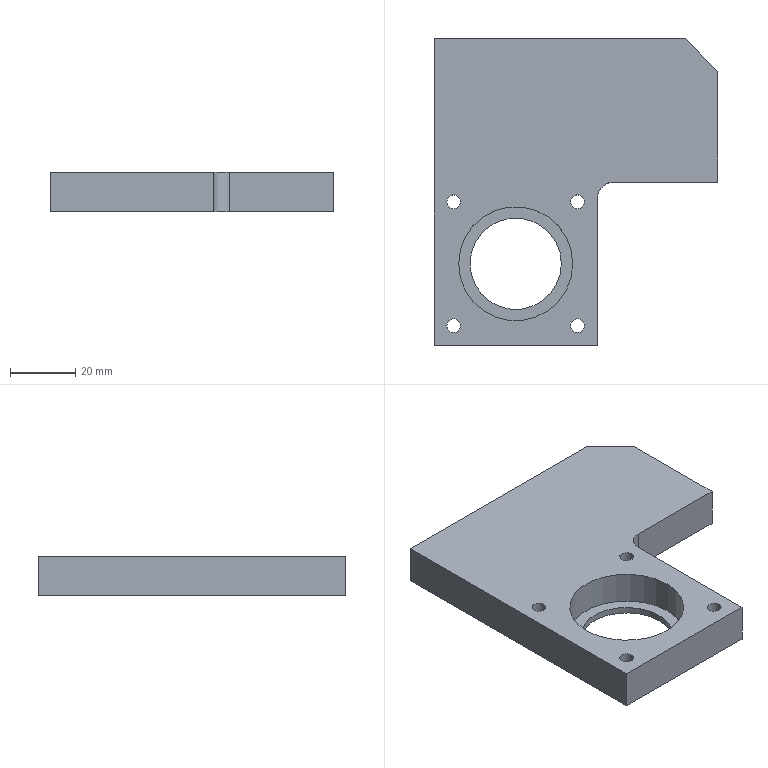Part | SolidWorks | features MirrorStock 1 | 1 solid | 47 faces | box 87 x 94 x 12 mm | volume 62817 mm3 | cylinder 25 | cone 12 | plane 10 | commonest cylinder face diameters 4.2 x20 28 x2 35 x2 10 x1
STEP:
#1=CARTESIAN_POINT('',(22.1,28.5,2.1));
#2=VERTEX_POINT('',#1);
#3=CARTESIAN_POINT('',(22.1,28.5,-2.1));
#4=VERTEX_POINT('',#3);
#5=CARTESIAN_POINT('',(22.1,28.5,0.));
#6=DIRECTION('',(-1.,0.,0.));
#7=DIRECTION('',(0.,0.,1.));
#8=AXIS2_PLACEMENT_3D('',#5,#6,#7);
#9=CIRCLE('',#8,2.1);
#10=EDGE_CURVE('',#2,#4,#9,.T.);
#11=ORIENTED_EDGE('',*,*,#10,.T.);
#12=CARTESIAN_POINT('',(34.5,28.5,-2.1));
#13=VERTEX_POINT('',#12);
#14=CARTESIAN_POINT('',(34.5,28.5,-2.1));
#15=DIRECTION('',(1.,0.,0.));
#16=VECTOR('',#15,1000.);
#17=LINE('',#14,#16);
#18=EDGE_CURVE('',#4,#13,#17,.T.);
#19=ORIENTED_EDGE('',*,*,#18,.T.);
#20=CARTESIAN_POINT('',(34.5,28.5,2.1));
#21=VERTEX_POINT('',#20);
#22=CARTESIAN_POINT('',(34.5,28.5,0.));
#23=DIRECTION('',(-1.,0.,0.));
#24=DIRECTION('',(0.,0.,1.));
#25=AXIS2_PLACEMENT_3D('',#22,#23,#24);
#26=CIRCLE('',#25,2.1);
#27=EDGE_CURVE('',#21,#13,#26,.T.);
#28=ORIENTED_EDGE('',*,*,#27,.F.);
#29=CARTESIAN_POINT('',(34.5,28.5,2.1));
#30=DIRECTION('',(1.,0.,0.));
#31=VECTOR('',#30,1000.);
#32=LINE('',#29,#31);
#33=EDGE_CURVE('',#2,#21,#32,.T.);
#34=ORIENTED_EDGE('',*,*,#33,.F.);
#35=EDGE_LOOP('',(#11,#19,#28,#34));
#36=FACE_OUTER_BOUND('',#35,.T.);
#37=CARTESIAN_POINT('',(34.5,28.5,0.));
#38=DIRECTION('',(1.,0.,0.));
#39=DIRECTION('',(0.,0.,1.));
#40=AXIS2_PLACEMENT_3D('',#37,#38,#39);
#41=CYLINDRICAL_SURFACE('',#40,2.1);
#42=ADVANCED_FACE('',(#36),#41,.F.);
#43=CARTESIAN_POINT('',(20.838,28.5,0.));
#44=VERTEX_POINT('',#43);
#45=CARTESIAN_POINT('',(22.1,28.5,2.1));
#46=DIRECTION('',(0.515,0.,0.8572));
#47=VECTOR('',#46,1000.);
#48=LINE('',#45,#47);
#49=EDGE_CURVE('',#44,#2,#48,.T.);
#50=ORIENTED_EDGE('',*,*,#49,.F.);
#51=CARTESIAN_POINT('',(22.1,28.5,-2.1));
#52=DIRECTION('',(0.515,0.,-0.8572));
#53=VECTOR('',#52,1000.);
#54=LINE('',#51,#53);
#55=EDGE_CURVE('',#44,#4,#54,.T.);
#56=ORIENTED_EDGE('',*,*,#55,.T.);
#57=ORIENTED_EDGE('',*,*,#10,.F.);
#58=EDGE_LOOP('',(#50,#56,#57));
#59=FACE_OUTER_BOUND('',#58,.T.);
#60=CARTESIAN_POINT('',(22.1,28.5,0.));
#61=DIRECTION('',(1.,0.,0.));
#62=DIRECTION('',(0.,0.,1.));
#63=AXIS2_PLACEMENT_3D('',#60,#61,#62);
#64=CONICAL_SURFACE('',#63,2.1,1.03);
#65=ADVANCED_FACE('',(#59),#64,.F.);
#66=CARTESIAN_POINT('',(22.1,10.5,2.1));
#67=VERTEX_POINT('',#66);
#68=CARTESIAN_POINT('',(22.1,10.5,-2.1));
#69=VERTEX_POINT('',#68);
#70=CARTESIAN_POINT('',(22.1,10.5,0.));
#71=DIRECTION('',(-1.,0.,0.));
#72=DIRECTION('',(0.,0.,1.));
#73=AXIS2_PLACEMENT_3D('',#70,#71,#72);
#74=CIRCLE('',#73,2.1);
#75=EDGE_CURVE('',#67,#69,#74,.T.);
#76=ORIENTED_EDGE('',*,*,#75,.T.);
#77=CARTESIAN_POINT('',(34.5,10.5,-2.1));
#78=VERTEX_POINT('',#77);
#79=CARTESIAN_POINT('',(34.5,10.5,-2.1));
#80=DIRECTION('',(1.,0.,0.));
#81=VECTOR('',#80,1000.);
#82=LINE('',#79,#81);
#83=EDGE_CURVE('',#69,#78,#82,.T.);
#84=ORIENTED_EDGE('',*,*,#83,.T.);
#85=CARTESIAN_POINT('',(34.5,10.5,2.1));
#86=VERTEX_POINT('',#85);
#87=CARTESIAN_POINT('',(34.5,10.5,0.));
#88=DIRECTION('',(-1.,0.,0.));
#89=DIRECTION('',(0.,0.,1.));
#90=AXIS2_PLACEMENT_3D('',#87,#88,#89);
#91=CIRCLE('',#90,2.1);
#92=EDGE_CURVE('',#86,#78,#91,.T.);
#93=ORIENTED_EDGE('',*,*,#92,.F.);
#94=CARTESIAN_POINT('',(34.5,10.5,2.1));
#95=DIRECTION('',(1.,0.,0.));
#96=VECTOR('',#95,1000.);
#97=LINE('',#94,#96);
#98=EDGE_CURVE('',#67,#86,#97,.T.);
#99=ORIENTED_EDGE('',*,*,#98,.F.);
#100=EDGE_LOOP('',(#76,#84,#93,#99));
#101=FACE_OUTER_BOUND('',#100,.T.);
#102=CARTESIAN_POINT('',(34.5,10.5,0.));
#103=DIRECTION('',(1.,0.,0.));
#104=DIRECTION('',(0.,0.,1.));
#105=AXIS2_PLACEMENT_3D('',#102,#103,#104);
#106=CYLINDRICAL_SURFACE('',#105,2.1);
#107=ADVANCED_FACE('',(#101),#106,.F.);
#108=CARTESIAN_POINT('',(20.838,10.5,0.));
#109=VERTEX_POINT('',#108);
#110=CARTESIAN_POINT('',(22.1,10.5,2.1));
#111=DIRECTION('',(0.515,0.,0.8572));
#112=VECTOR('',#111,1000.);
#113=LINE('',#110,#112);
#114=EDGE_CURVE('',#109,#67,#113,.T.);
#115=ORIENTED_EDGE('',*,*,#114,.F.);
#116=CARTESIAN_POINT('',(22.1,10.5,-2.1));
#117=DIRECTION('',(0.515,0.,-0.8572));
#118=VECTOR('',#117,1000.);
#119=LINE('',#116,#118);
#120=EDGE_CURVE('',#109,#69,#119,.T.);
#121=ORIENTED_EDGE('',*,*,#120,.T.);
#122=ORIENTED_EDGE('',*,*,#75,.F.);
#123=EDGE_LOOP('',(#115,#121,#122));
#124=FACE_OUTER_BOUND('',#123,.T.);
#125=CARTESIAN_POINT('',(22.1,10.5,0.));
#126=DIRECTION('',(1.,0.,0.));
#127=DIRECTION('',(0.,0.,1.));
#128=AXIS2_PLACEMENT_3D('',#125,#126,#127);
#129=CONICAL_SURFACE('',#128,2.1,1.03);
#130=ADVANCED_FACE('',(#124),#129,.F.);
#131=CARTESIAN_POINT('',(12.5,34.1,-2.1));
#132=VERTEX_POINT('',#131);
#133=CARTESIAN_POINT('',(12.5,34.1,2.1));
#134=VERTEX_POINT('',#133);
#135=CARTESIAN_POINT('',(12.5,34.1,0.));
#136=DIRECTION('',(0.,-1.,0.));
#137=DIRECTION('',(0.,0.,-1.));
#138=AXIS2_PLACEMENT_3D('',#135,#136,#137);
#139=CIRCLE('',#138,2.1);
#140=EDGE_CURVE('',#132,#134,#139,.T.);
#141=ORIENTED_EDGE('',*,*,#140,.T.);
#142=CARTESIAN_POINT('',(12.5,46.5,2.1));
#143=VERTEX_POINT('',#142);
#144=CARTESIAN_POINT('',(12.5,46.5,2.1));
#145=DIRECTION('',(0.,1.,0.));
#146=VECTOR('',#145,1000.);
#147=LINE('',#144,#146);
#148=EDGE_CURVE('',#134,#143,#147,.T.);
#149=ORIENTED_EDGE('',*,*,#148,.T.);
#150=CARTESIAN_POINT('',(12.5,46.5,-2.1));
#151=VERTEX_POINT('',#150);
#152=CARTESIAN_POINT('',(12.5,46.5,0.));
#153=DIRECTION('',(0.,-1.,0.));
#154=DIRECTION('',(0.,0.,-1.));
#155=AXIS2_PLACEMENT_3D('',#152,#153,#154);
#156=CIRCLE('',#155,2.1);
#157=EDGE_CURVE('',#151,#143,#156,.T.);
#158=ORIENTED_EDGE('',*,*,#157,.F.);
#159=CARTESIAN_POINT('',(12.5,46.5,-2.1));
#160=DIRECTION('',(0.,1.,0.));
#161=VECTOR('',#160,1000.);
#162=LINE('',#159,#161);
#163=EDGE_CURVE('',#132,#151,#162,.T.);
#164=ORIENTED_EDGE('',*,*,#163,.F.);
#165=EDGE_LOOP('',(#141,#149,#158,#164));
#166=FACE_OUTER_BOUND('',#165,.T.);
#167=CARTESIAN_POINT('',(12.5,46.5,0.));
#168=DIRECTION('',(0.,1.,0.));
#169=DIRECTION('',(0.,0.,-1.));
#170=AXIS2_PLACEMENT_3D('',#167,#168,#169);
#171=CYLINDRICAL_SURFACE('',#170,2.1);
#172=ADVANCED_FACE('',(#166),#171,.F.);
#173=CARTESIAN_POINT('',(12.5,32.838,0.));
#174=VERTEX_POINT('',#173);
#175=CARTESIAN_POINT('',(12.5,34.1,-2.1));
#176=DIRECTION('',(0.,0.515,-0.8572));
#177=VECTOR('',#176,1000.);
#178=LINE('',#175,#177);
#179=EDGE_CURVE('',#174,#132,#178,.T.);
#180=ORIENTED_EDGE('',*,*,#179,.F.);
#181=CARTESIAN_POINT('',(12.5,34.1,2.1));
#182=DIRECTION('',(0.,0.515,0.8572));
#183=VECTOR('',#182,1000.);
#184=LINE('',#181,#183);
#185=EDGE_CURVE('',#174,#134,#184,.T.);
#186=ORIENTED_EDGE('',*,*,#185,.T.);
#187=ORIENTED_EDGE('',*,*,#140,.F.);
#188=EDGE_LOOP('',(#180,#186,#187));
#189=FACE_OUTER_BOUND('',#188,.T.);
#190=CARTESIAN_POINT('',(12.5,34.1,0.));
#191=DIRECTION('',(0.,1.,0.));
#192=DIRECTION('',(0.,0.,-1.));
#193=AXIS2_PLACEMENT_3D('',#190,#191,#192);
#194=CONICAL_SURFACE('',#193,2.1,1.03);
#195=ADVANCED_FACE('',(#189),#194,.F.);
#196=CARTESIAN_POINT('',(-7.5,34.1,-2.1));
#197=VERTEX_POINT('',#196);
#198=CARTESIAN_POINT('',(-7.5,34.1,2.1));
#199=VERTEX_POINT('',#198);
#200=CARTESIAN_POINT('',(-7.5,34.1,0.));
#201=DIRECTION('',(0.,-1.,0.));
#202=DIRECTION('',(0.,0.,-1.));
#203=AXIS2_PLACEMENT_3D('',#200,#201,#202);
#204=CIRCLE('',#203,2.1);
#205=EDGE_CURVE('',#197,#199,#204,.T.);
#206=ORIENTED_EDGE('',*,*,#205,.T.);
#207=CARTESIAN_POINT('',(-7.5,46.5,2.1));
#208=VERTEX_POINT('',#207);
#209=CARTESIAN_POINT('',(-7.5,46.5,2.1));
#210=DIRECTION('',(0.,1.,0.));
#211=VECTOR('',#210,1000.);
#212=LINE('',#209,#211);
#213=EDGE_CURVE('',#199,#208,#212,.T.);
#214=ORIENTED_EDGE('',*,*,#213,.T.);
#215=CARTESIAN_POINT('',(-7.5,46.5,-2.1));
#216=VERTEX_POINT('',#215);
#217=CARTESIAN_POINT('',(-7.5,46.5,0.));
#218=DIRECTION('',(0.,-1.,0.));
#219=DIRECTION('',(0.,0.,-1.));
#220=AXIS2_PLACEMENT_3D('',#217,#218,#219);
#221=CIRCLE('',#220,2.1);
#222=EDGE_CURVE('',#216,#208,#221,.T.);
#223=ORIENTED_EDGE('',*,*,#222,.F.);
#224=CARTESIAN_POINT('',(-7.5,46.5,-2.1));
#225=DIRECTION('',(0.,1.,0.));
#226=VECTOR('',#225,1000.);
#227=LINE('',#224,#226);
#228=EDGE_CURVE('',#197,#216,#227,.T.);
#229=ORIENTED_EDGE('',*,*,#228,.F.);
#230=EDGE_LOOP('',(#206,#214,#223,#229));
#231=FACE_OUTER_BOUND('',#230,.T.);
#232=CARTESIAN_POINT('',(-7.5,46.5,0.));
#233=DIRECTION('',(0.,1.,0.));
#234=DIRECTION('',(0.,0.,-1.));
#235=AXIS2_PLACEMENT_3D('',#232,#233,#234);
#236=CYLINDRICAL_SURFACE('',#235,2.1);
#237=ADVANCED_FACE('',(#231),#236,.F.);
#238=CARTESIAN_POINT('',(-7.5,32.838,0.));
#239=VERTEX_POINT('',#238);
#240=CARTESIAN_POINT('',(-7.5,34.1,-2.1));
#241=DIRECTION('',(0.,0.515,-0.8572));
#242=VECTOR('',#241,1000.);
#243=LINE('',#240,#242);
#244=EDGE_CURVE('',#239,#197,#243,.T.);
#245=ORIENTED_EDGE('',*,*,#244,.F.);
#246=CARTESIAN_POINT('',(-7.5,34.1,2.1));
#247=DIRECTION('',(0.,0.515,0.8572));
#248=VECTOR('',#247,1000.);
#249=LINE('',#246,#248);
#250=EDGE_CURVE('',#239,#199,#249,.T.);
#251=ORIENTED_EDGE('',*,*,#250,.T.);
#252=ORIENTED_EDGE('',*,*,#205,.F.);
#253=EDGE_LOOP('',(#245,#251,#252));
#254=FACE_OUTER_BOUND('',#253,.T.);
#255=CARTESIAN_POINT('',(-7.5,34.1,0.));
#256=DIRECTION('',(0.,1.,0.));
#257=DIRECTION('',(0.,0.,-1.));
#258=AXIS2_PLACEMENT_3D('',#255,#256,#257);
#259=CONICAL_SURFACE('',#258,2.1,1.03);
#260=ADVANCED_FACE('',(#254),#259,.F.);
#261=CARTESIAN_POINT('',(-27.5,34.1,-2.1));
#262=VERTEX_POINT('',#261);
#263=CARTESIAN_POINT('',(-27.5,34.1,2.1));
#264=VERTEX_POINT('',#263);
#265=CARTESIAN_POINT('',(-27.5,34.1,0.));
#266=DIRECTION('',(0.,-1.,0.));
#267=DIRECTION('',(0.,0.,-1.));
#268=AXIS2_PLACEMENT_3D('',#265,#266,#267);
#269=CIRCLE('',#268,2.1);
#270=EDGE_CURVE('',#262,#264,#269,.T.);
#271=ORIENTED_EDGE('',*,*,#270,.T.);
#272=CARTESIAN_POINT('',(-27.5,46.5,2.1));
#273=VERTEX_POINT('',#272);
#274=CARTESIAN_POINT('',(-27.5,46.5,2.1));
#275=DIRECTION('',(0.,1.,0.));
#276=VECTOR('',#275,1000.);
#277=LINE('',#274,#276);
#278=EDGE_CURVE('',#264,#273,#277,.T.);
#279=ORIENTED_EDGE('',*,*,#278,.T.);
#280=CARTESIAN_POINT('',(-27.5,46.5,-2.1));
#281=VERTEX_POINT('',#280);
#282=CARTESIAN_POINT('',(-27.5,46.5,0.));
#283=DIRECTION('',(0.,-1.,0.));
#284=DIRECTION('',(0.,0.,-1.));
#285=AXIS2_PLACEMENT_3D('',#282,#283,#284);
#286=CIRCLE('',#285,2.1);
#287=EDGE_CURVE('',#281,#273,#286,.T.);
#288=ORIENTED_EDGE('',*,*,#287,.F.);
#289=CARTESIAN_POINT('',(-27.5,46.5,-2.1));
#290=DIRECTION('',(0.,1.,0.));
#291=VECTOR('',#290,1000.);
#292=LINE('',#289,#291);
#293=EDGE_CURVE('',#262,#281,#292,.T.);
#294=ORIENTED_EDGE('',*,*,#293,.F.);
#295=EDGE_LOOP('',(#271,#279,#288,#294));
#296=FACE_OUTER_BOUND('',#295,.T.);
#297=CARTESIAN_POINT('',(-27.5,46.5,0.));
#298=DIRECTION('',(0.,1.,0.));
#299=DIRECTION('',(0.,0.,-1.));
#300=AXIS2_PLACEMENT_3D('',#297,#298,#299);
#301=CYLINDRICAL_SURFACE('',#300,2.1);
#302=ADVANCED_FACE('',(#296),#301,.F.);
#303=CARTESIAN_POINT('',(-27.5,32.838,0.));
#304=VERTEX_POINT('',#303);
#305=CARTESIAN_POINT('',(-27.5,34.1,-2.1));
#306=DIRECTION('',(0.,0.515,-0.8572));
#307=VECTOR('',#306,1000.);
#308=LINE('',#305,#307);
#309=EDGE_CURVE('',#304,#262,#308,.T.);
#310=ORIENTED_EDGE('',*,*,#309,.F.);
#311=CARTESIAN_POINT('',(-27.5,34.1,2.1));
#312=DIRECTION('',(0.,0.515,0.8572));
#313=VECTOR('',#312,1000.);
#314=LINE('',#311,#313);
#315=EDGE_CURVE('',#304,#264,#314,.T.);
#316=ORIENTED_EDGE('',*,*,#315,.T.);
#317=ORIENTED_EDGE('',*,*,#270,.F.);
#318=EDGE_LOOP('',(#310,#316,#317));
#319=FACE_OUTER_BOUND('',#318,.T.);
#320=CARTESIAN_POINT('',(-27.5,34.1,0.));
#321=DIRECTION('',(0.,1.,0.));
#322=DIRECTION('',(0.,0.,-1.));
#323=AXIS2_PLACEMENT_3D('',#320,#321,#322);
#324=CONICAL_SURFACE('',#323,2.1,1.03);
#325=ADVANCED_FACE('',(#319),#324,.F.);
#326=CARTESIAN_POINT('',(-47.5,34.1,-2.1));
#327=VERTEX_POINT('',#326);
#328=CARTESIAN_POINT('',(-47.5,34.1,2.1));
#329=VERTEX_POINT('',#328);
#330=CARTESIAN_POINT('',(-47.5,34.1,0.));
#331=DIRECTION('',(0.,-1.,0.));
#332=DIRECTION('',(0.,0.,-1.));
#333=AXIS2_PLACEMENT_3D('',#330,#331,#332);
#334=CIRCLE('',#333,2.1);
#335=EDGE_CURVE('',#327,#329,#334,.T.);
#336=ORIENTED_EDGE('',*,*,#335,.T.);
#337=CARTESIAN_POINT('',(-47.5,46.5,2.1));
#338=VERTEX_POINT('',#337);
#339=CARTESIAN_POINT('',(-47.5,46.5,2.1));
#340=DIRECTION('',(0.,1.,0.));
#341=VECTOR('',#340,1000.);
#342=LINE('',#339,#341);
#343=EDGE_CURVE('',#329,#338,#342,.T.);
#344=ORIENTED_EDGE('',*,*,#343,.T.);
#345=CARTESIAN_POINT('',(-47.5,46.5,-2.1));
#346=VERTEX_POINT('',#345);
#347=CARTESIAN_POINT('',(-47.5,46.5,0.));
#348=DIRECTION('',(0.,-1.,0.));
#349=DIRECTION('',(0.,0.,-1.));
#350=AXIS2_PLACEMENT_3D('',#347,#348,#349);
#351=CIRCLE('',#350,2.1);
#352=EDGE_CURVE('',#346,#338,#351,.T.);
#353=ORIENTED_EDGE('',*,*,#352,.F.);
#354=CARTESIAN_POINT('',(-47.5,46.5,-2.1));
#355=DIRECTION('',(0.,1.,0.));
#356=VECTOR('',#355,1000.);
#357=LINE('',#354,#356);
#358=EDGE_CURVE('',#327,#346,#357,.T.);
#359=ORIENTED_EDGE('',*,*,#358,.F.);
#360=EDGE_LOOP('',(#336,#344,#353,#359));
#361=FACE_OUTER_BOUND('',#360,.T.);
#362=CARTESIAN_POINT('',(-47.5,46.5,0.));
#363=DIRECTION('',(0.,1.,0.));
#364=DIRECTION('',(0.,0.,-1.));
#365=AXIS2_PLACEMENT_3D('',#362,#363,#364);
#366=CYLINDRICAL_SURFACE('',#365,2.1);
#367=ADVANCED_FACE('',(#361),#366,.F.);
#368=CARTESIAN_POINT('',(-47.5,32.838,0.));
#369=VERTEX_POINT('',#368);
#370=CARTESIAN_POINT('',(-47.5,34.1,-2.1));
#371=DIRECTION('',(0.,0.515,-0.8572));
#372=VECTOR('',#371,1000.);
#373=LINE('',#370,#372);
#374=EDGE_CURVE('',#369,#327,#373,.T.);
#375=ORIENTED_EDGE('',*,*,#374,.F.);
#376=CARTESIAN_POINT('',(-47.5,34.1,2.1));
#377=DIRECTION('',(0.,0.515,0.8572));
#378=VECTOR('',#377,1000.);
#379=LINE('',#376,#378);
#380=EDGE_CURVE('',#369,#329,#379,.T.);
#381=ORIENTED_EDGE('',*,*,#380,.T.);
#382=ORIENTED_EDGE('',*,*,#335,.F.);
#383=EDGE_LOOP('',(#375,#381,#382));
#384=FACE_OUTER_BOUND('',#383,.T.);
#385=CARTESIAN_POINT('',(-47.5,34.1,0.));
#386=DIRECTION('',(0.,1.,0.));
#387=DIRECTION('',(0.,0.,-1.));
#388=AXIS2_PLACEMENT_3D('',#385,#386,#387);
#389=CONICAL_SURFACE('',#388,2.1,1.03);
#390=ADVANCED_FACE('',(#384),#389,.F.);
#391=CARTESIAN_POINT('',(-10.6,-3.5,-6.));
#392=VERTEX_POINT('',#391);
#393=CARTESIAN_POINT('',(-6.4,-3.5,-6.));
#394=VERTEX_POINT('',#393);
#395=CARTESIAN_POINT('',(-8.5,-3.5,-6.));
#396=DIRECTION('',(0.,0.,-1.));
#397=DIRECTION('',(-1.,0.,0.));
#398=AXIS2_PLACEMENT_3D('',#395,#396,#397);
#399=CIRCLE('',#398,2.1);
#400=EDGE_CURVE('',#392,#394,#399,.T.);
#401=ORIENTED_EDGE('',*,*,#400,.T.);
#402=CARTESIAN_POINT('',(-6.4,-3.5,6.));
#403=VERTEX_POINT('',#402);
#404=CARTESIAN_POINT('',(-6.4,-3.5,6.));
#405=DIRECTION('',(0.,0.,1.));
#406=VECTOR('',#405,1000.);
#407=LINE('',#404,#406);
#408=EDGE_CURVE('',#394,#403,#407,.T.);
#409=ORIENTED_EDGE('',*,*,#408,.T.);
#410=CARTESIAN_POINT('',(-10.6,-3.5,6.));
#411=VERTEX_POINT('',#410);
#412=CARTESIAN_POINT('',(-8.5,-3.5,6.));
#413=DIRECTION('',(0.,0.,-1.));
#414=DIRECTION('',(-1.,0.,0.));
#415=AXIS2_PLACEMENT_3D('',#412,#413,#414);
#416=CIRCLE('',#415,2.1);
#417=EDGE_CURVE('',#411,#403,#416,.T.);
#418=ORIENTED_EDGE('',*,*,#417,.F.);
#419=CARTESIAN_POINT('',(-10.6,-3.5,6.));
#420=DIRECTION('',(0.,0.,1.));
#421=VECTOR('',#420,1000.);
#422=LINE('',#419,#421);
#423=EDGE_CURVE('',#392,#411,#422,.T.);
#424=ORIENTED_EDGE('',*,*,#423,.F.);
#425=EDGE_LOOP('',(#401,#409,#418,#424));
#426=FACE_OUTER_BOUND('',#425,.T.);
#427=CARTESIAN_POINT('',(-8.5,-3.5,6.));
#428=DIRECTION('',(0.,0.,1.));
#429=DIRECTION('',(-1.,0.,0.));
#430=AXIS2_PLACEMENT_3D('',#427,#428,#429);
#431=CYLINDRICAL_SURFACE('',#430,2.1);
#432=ADVANCED_FACE('',(#426),#431,.F.);
#433=CARTESIAN_POINT('',(-10.6,-41.5,-6.));
#434=VERTEX_POINT('',#433);
#435=CARTESIAN_POINT('',(-6.4,-41.5,-6.));
#436=VERTEX_POINT('',#435);
#437=CARTESIAN_POINT('',(-8.5,-41.5,-6.));
#438=DIRECTION('',(0.,0.,-1.));
#439=DIRECTION('',(-1.,0.,0.));
#440=AXIS2_PLACEMENT_3D('',#437,#438,#439);
#441=CIRCLE('',#440,2.1);
#442=EDGE_CURVE('',#434,#436,#441,.T.);
#443=ORIENTED_EDGE('',*,*,#442,.T.);
#444=CARTESIAN_POINT('',(-6.4,-41.5,6.));
#445=VERTEX_POINT('',#444);
#446=CARTESIAN_POINT('',(-6.4,-41.5,6.));
#447=DIRECTION('',(0.,0.,1.));
#448=VECTOR('',#447,1000.);
#449=LINE('',#446,#448);
#450=EDGE_CURVE('',#436,#445,#449,.T.);
#451=ORIENTED_EDGE('',*,*,#450,.T.);
#452=CARTESIAN_POINT('',(-10.6,-41.5,6.));
#453=VERTEX_POINT('',#452);
#454=CARTESIAN_POINT('',(-8.5,-41.5,6.));
#455=DIRECTION('',(0.,0.,-1.));
#456=DIRECTION('',(-1.,0.,0.));
#457=AXIS2_PLACEMENT_3D('',#454,#455,#456);
#458=CIRCLE('',#457,2.1);
#459=EDGE_CURVE('',#453,#445,#458,.T.);
#460=ORIENTED_EDGE('',*,*,#459,.F.);
#461=CARTESIAN_POINT('',(-10.6,-41.5,6.));
#462=DIRECTION('',(0.,0.,1.));
#463=VECTOR('',#462,1000.);
#464=LINE('',#461,#463);
#465=EDGE_CURVE('',#434,#453,#464,.T.);
#466=ORIENTED_EDGE('',*,*,#465,.F.);
#467=EDGE_LOOP('',(#443,#451,#460,#466));
#468=FACE_OUTER_BOUND('',#467,.T.);
#469=CARTESIAN_POINT('',(-8.5,-41.5,6.));
#470=DIRECTION('',(0.,0.,1.));
#471=DIRECTION('',(-1.,0.,0.));
#472=AXIS2_PLACEMENT_3D('',#469,#470,#471);
#473=CYLINDRICAL_SURFACE('',#472,2.1);
#474=ADVANCED_FACE('',(#468),#473,.F.);
#475=CARTESIAN_POINT('',(-48.6,-41.5,-6.));
#476=VERTEX_POINT('',#475);
#477=CARTESIAN_POINT('',(-44.4,-41.5,-6.));
#478=VERTEX_POINT('',#477);
#479=CARTESIAN_POINT('',(-46.5,-41.5,-6.));
#480=DIRECTION('',(0.,0.,-1.));
#481=DIRECTION('',(-1.,0.,0.));
#482=AXIS2_PLACEMENT_3D('',#479,#480,#481);
#483=CIRCLE('',#482,2.1);
#484=EDGE_CURVE('',#476,#478,#483,.T.);
#485=ORIENTED_EDGE('',*,*,#484,.T.);
#486=CARTESIAN_POINT('',(-44.4,-41.5,6.));
#487=VERTEX_POINT('',#486);
#488=CARTESIAN_POINT('',(-44.4,-41.5,6.));
#489=DIRECTION('',(0.,0.,1.));
#490=VECTOR('',#489,1000.);
#491=LINE('',#488,#490);
#492=EDGE_CURVE('',#478,#487,#491,.T.);
#493=ORIENTED_EDGE('',*,*,#492,.T.);
#494=CARTESIAN_POINT('',(-48.6,-41.5,6.));
#495=VERTEX_POINT('',#494);
#496=CARTESIAN_POINT('',(-46.5,-41.5,6.));
#497=DIRECTION('',(0.,0.,-1.));
#498=DIRECTION('',(-1.,0.,0.));
#499=AXIS2_PLACEMENT_3D('',#496,#497,#498);
#500=CIRCLE('',#499,2.1);
#501=EDGE_CURVE('',#495,#487,#500,.T.);
#502=ORIENTED_EDGE('',*,*,#501,.F.);
#503=CARTESIAN_POINT('',(-48.6,-41.5,6.));
#504=DIRECTION('',(0.,0.,1.));
#505=VECTOR('',#504,1000.);
#506=LINE('',#503,#505);
#507=EDGE_CURVE('',#476,#495,#506,.T.);
#508=ORIENTED_EDGE('',*,*,#507,.F.);
#509=EDGE_LOOP('',(#485,#493,#502,#508));
#510=FACE_OUTER_BOUND('',#509,.T.);
#511=CARTESIAN_POINT('',(-46.5,-41.5,6.));
#512=DIRECTION('',(0.,0.,1.));
#513=DIRECTION('',(-1.,0.,0.));
#514=AXIS2_PLACEMENT_3D('',#511,#512,#513);
#515=CYLINDRICAL_SURFACE('',#514,2.1);
#516=ADVANCED_FACE('',(#510),#515,.F.);
#517=CARTESIAN_POINT('',(-48.6,-3.5,-6.));
#518=VERTEX_POINT('',#517);
#519=CARTESIAN_POINT('',(-44.4,-3.5,-6.));
#520=VERTEX_POINT('',#519);
#521=CARTESIAN_POINT('',(-46.5,-3.5,-6.));
#522=DIRECTION('',(0.,0.,-1.));
#523=DIRECTION('',(-1.,0.,0.));
#524=AXIS2_PLACEMENT_3D('',#521,#522,#523);
#525=CIRCLE('',#524,2.1);
#526=EDGE_CURVE('',#518,#520,#525,.T.);
#527=ORIENTED_EDGE('',*,*,#526,.T.);
#528=CARTESIAN_POINT('',(-44.4,-3.5,6.));
#529=VERTEX_POINT('',#528);
#530=CARTESIAN_POINT('',(-44.4,-3.5,6.));
#531=DIRECTION('',(0.,0.,1.));
#532=VECTOR('',#531,1000.);
#533=LINE('',#530,#532);
#534=EDGE_CURVE('',#520,#529,#533,.T.);
#535=ORIENTED_EDGE('',*,*,#534,.T.);
#536=CARTESIAN_POINT('',(-48.6,-3.5,6.));
#537=VERTEX_POINT('',#536);
#538=CARTESIAN_POINT('',(-46.5,-3.5,6.));
#539=DIRECTION('',(0.,0.,-1.));
#540=DIRECTION('',(-1.,0.,0.));
#541=AXIS2_PLACEMENT_3D('',#538,#539,#540);
#542=CIRCLE('',#541,2.1);
#543=EDGE_CURVE('',#537,#529,#542,.T.);
#544=ORIENTED_EDGE('',*,*,#543,.F.);
#545=CARTESIAN_POINT('',(-48.6,-3.5,6.));
#546=DIRECTION('',(0.,0.,1.));
#547=VECTOR('',#546,1000.);
#548=LINE('',#545,#547);
#549=EDGE_CURVE('',#518,#537,#548,.T.);
#550=ORIENTED_EDGE('',*,*,#549,.F.);
#551=EDGE_LOOP('',(#527,#535,#544,#550));
#552=FACE_OUTER_BOUND('',#551,.T.);
#553=CARTESIAN_POINT('',(-46.5,-3.5,6.));
#554=DIRECTION('',(0.,0.,1.));
#555=DIRECTION('',(-1.,0.,0.));
#556=AXIS2_PLACEMENT_3D('',#553,#554,#555);
#557=CYLINDRICAL_SURFACE('',#556,2.1);
#558=ADVANCED_FACE('',(#552),#557,.F.);
#559=CARTESIAN_POINT('',(-41.5,-22.5,-6.));
#560=VERTEX_POINT('',#559);
#561=CARTESIAN_POINT('',(-13.5,-22.5,-6.));
#562=VERTEX_POINT('',#561);
#563=CARTESIAN_POINT('',(-27.5,-22.5,-6.));
#564=DIRECTION('',(0.,0.,-1.));
#565=DIRECTION('',(-1.,0.,0.));
#566=AXIS2_PLACEMENT_3D('',#563,#564,#565);
#567=CIRCLE('',#566,14.);
#568=EDGE_CURVE('',#560,#562,#567,.T.);
#569=ORIENTED_EDGE('',*,*,#568,.T.);
#570=CARTESIAN_POINT('',(-13.5,-22.5,-4.));
#571=VERTEX_POINT('',#570);
#572=CARTESIAN_POINT('',(-13.5,-22.5,-6.));
#573=DIRECTION('',(0.,0.,1.));
#574=VECTOR('',#573,1000.);
#575=LINE('',#572,#574);
#576=EDGE_CURVE('',#562,#571,#575,.T.);
#577=ORIENTED_EDGE('',*,*,#576,.T.);
#578=CARTESIAN_POINT('',(-41.5,-22.5,-4.));
#579=VERTEX_POINT('',#578);
#580=CARTESIAN_POINT('',(-27.5,-22.5,-4.));
#581=DIRECTION('',(0.,0.,-1.));
#582=DIRECTION('',(-1.,0.,0.));
#583=AXIS2_PLACEMENT_3D('',#580,#581,#582);
#584=CIRCLE('',#583,14.);
#585=EDGE_CURVE('',#579,#571,#584,.T.);
#586=ORIENTED_EDGE('',*,*,#585,.F.);
#587=CARTESIAN_POINT('',(-41.5,-22.5,-6.));
#588=DIRECTION('',(0.,0.,1.));
#589=VECTOR('',#588,1000.);
#590=LINE('',#587,#589);
#591=EDGE_CURVE('',#560,#579,#590,.T.);
#592=ORIENTED_EDGE('',*,*,#591,.F.);
#593=EDGE_LOOP('',(#569,#577,#586,#592));
#594=FACE_OUTER_BOUND('',#593,.T.);
#595=CARTESIAN_POINT('',(-27.5,-22.5,-6.));
#596=DIRECTION('',(0.,0.,1.));
#597=DIRECTION('',(-1.,0.,0.));
#598=AXIS2_PLACEMENT_3D('',#595,#596,#597);
#599=CYLINDRICAL_SURFACE('',#598,14.);
#600=ADVANCED_FACE('',(#594),#599,.F.);
#601=CARTESIAN_POINT('',(-10.,-22.5,-4.));
#602=VERTEX_POINT('',#601);
#603=CARTESIAN_POINT('',(-45.,-22.5,-4.));
#604=VERTEX_POINT('',#603);
#605=CARTESIAN_POINT('',(-27.5,-22.5,-4.));
#606=DIRECTION('',(0.,0.,1.));
#607=DIRECTION('',(1.,0.,0.));
#608=AXIS2_PLACEMENT_3D('',#605,#606,#607);
#609=CIRCLE('',#608,17.5);
#610=EDGE_CURVE('',#602,#604,#609,.T.);
#611=ORIENTED_EDGE('',*,*,#610,.F.);
#612=CARTESIAN_POINT('',(-10.,-22.5,6.));
#613=VERTEX_POINT('',#612);
#614=CARTESIAN_POINT('',(-10.,-22.5,-4.));
#615=DIRECTION('',(0.,0.,1.));
#616=VECTOR('',#615,1000.);
#617=LINE('',#614,#616);
#618=EDGE_CURVE('',#602,#613,#617,.T.);
#619=ORIENTED_EDGE('',*,*,#618,.T.);
#620=CARTESIAN_POINT('',(-45.,-22.5,6.));
#621=VERTEX_POINT('',#620);
#622=CARTESIAN_POINT('',(-27.5,-22.5,6.));
#623=DIRECTION('',(0.,0.,1.));
#624=DIRECTION('',(1.,0.,0.));
#625=AXIS2_PLACEMENT_3D('',#622,#623,#624);
#626=CIRCLE('',#625,17.5);
#627=EDGE_CURVE('',#613,#621,#626,.T.);
#628=ORIENTED_EDGE('',*,*,#627,.T.);
#629=CARTESIAN_POINT('',(-45.,-22.5,-4.));
#630=DIRECTION('',(0.,0.,1.));
#631=VECTOR('',#630,1000.);
#632=LINE('',#629,#631);
#633=EDGE_CURVE('',#604,#621,#632,.T.);
#634=ORIENTED_EDGE('',*,*,#633,.F.);
#635=EDGE_LOOP('',(#611,#619,#628,#634));
#636=FACE_OUTER_BOUND('',#635,.T.);
#637=CARTESIAN_POINT('',(-27.5,-22.5,-4.));
#638=DIRECTION('',(0.,0.,1.));
#639=DIRECTION('',(-1.,0.,0.));
#640=AXIS2_PLACEMENT_3D('',#637,#638,#639);
#641=CYLINDRICAL_SURFACE('',#640,17.5);
#642=ADVANCED_FACE('',(#636),#641,.F.);
#643=ORIENTED_EDGE('',*,*,#27,.T.);
#644=CARTESIAN_POINT('',(34.5,28.5,0.));
#645=DIRECTION('',(-1.,0.,0.));
#646=DIRECTION('',(0.,0.,1.));
#647=AXIS2_PLACEMENT_3D('',#644,#645,#646);
#648=CIRCLE('',#647,2.1);
#649=EDGE_CURVE('',#13,#21,#648,.T.);
#650=ORIENTED_EDGE('',*,*,#649,.T.);
#651=EDGE_LOOP('',(#643,#650));
#652=FACE_BOUND('',#651,.T.);
#653=ORIENTED_EDGE('',*,*,#92,.T.);
#654=CARTESIAN_POINT('',(34.5,10.5,0.));
#655=DIRECTION('',(-1.,0.,0.));
#656=DIRECTION('',(0.,0.,1.));
#657=AXIS2_PLACEMENT_3D('',#654,#655,#656);
#658=CIRCLE('',#657,2.1);
#659=EDGE_CURVE('',#78,#86,#658,.T.);
#660=ORIENTED_EDGE('',*,*,#659,.T.);
#661=EDGE_LOOP('',(#653,#660));
#662=FACE_BOUND('',#661,.T.);
#663=CARTESIAN_POINT('',(34.5,2.5,6.));
#664=VERTEX_POINT('',#663);
#665=CARTESIAN_POINT('',(34.5,36.5,6.));
#666=VERTEX_POINT('',#665);
#667=CARTESIAN_POINT('',(34.5,-47.5,6.));
#668=DIRECTION('',(0.,1.,0.));
#669=VECTOR('',#668,1000.);
#670=LINE('',#667,#669);
#671=EDGE_CURVE('',#664,#666,#670,.T.);
#672=ORIENTED_EDGE('',*,*,#671,.F.);
#673=CARTESIAN_POINT('',(34.5,2.5,-6.));
#674=VERTEX_POINT('',#673);
#675=CARTESIAN_POINT('',(34.5,2.5,6.));
#676=DIRECTION('',(0.,0.,-1.));
#677=VECTOR('',#676,1000.);
#678=LINE('',#675,#677);
#679=EDGE_CURVE('',#664,#674,#678,.T.);
#680=ORIENTED_EDGE('',*,*,#679,.T.);
#681=CARTESIAN_POINT('',(34.5,36.5,-6.));
#682=VERTEX_POINT('',#681);
#683=CARTESIAN_POINT('',(34.5,-47.5,-6.));
#684=DIRECTION('',(0.,1.,0.));
#685=VECTOR('',#684,1000.);
#686=LINE('',#683,#685);
#687=EDGE_CURVE('',#674,#682,#686,.T.);
#688=ORIENTED_EDGE('',*,*,#687,.T.);
#689=CARTESIAN_POINT('',(34.5,36.5,-6.));
#690=DIRECTION('',(0.,0.,-1.));
#691=VECTOR('',#690,1000.);
#692=LINE('',#689,#691);
#693=EDGE_CURVE('',#666,#682,#692,.T.);
#694=ORIENTED_EDGE('',*,*,#693,.F.);
#695=EDGE_LOOP('',(#672,#680,#688,#694));
#696=FACE_OUTER_BOUND('',#695,.T.);
#697=CARTESIAN_POINT('',(34.5,-47.5,-6.));
#698=DIRECTION('',(-1.,0.,0.));
#699=DIRECTION('',(0.,0.,-1.));
#700=AXIS2_PLACEMENT_3D('',#697,#698,#699);
#701=PLANE('',#700);
#702=ADVANCED_FACE('',(#652,#662,#696),#701,.F.);
#703=ORIENTED_EDGE('',*,*,#157,.T.);
#704=CARTESIAN_POINT('',(12.5,46.5,0.));
#705=DIRECTION('',(0.,-1.,0.));
#706=DIRECTION('',(0.,0.,-1.));
#707=AXIS2_PLACEMENT_3D('',#704,#705,#706);
#708=CIRCLE('',#707,2.1);
#709=EDGE_CURVE('',#143,#151,#708,.T.);
#710=ORIENTED_EDGE('',*,*,#709,.T.);
#711=EDGE_LOOP('',(#703,#710));
#712=FACE_BOUND('',#711,.T.);
#713=ORIENTED_EDGE('',*,*,#222,.T.);
#714=CARTESIAN_POINT('',(-7.5,46.5,0.));
#715=DIRECTION('',(0.,-1.,0.));
#716=DIRECTION('',(0.,0.,-1.));
#717=AXIS2_PLACEMENT_3D('',#714,#715,#716);
#718=CIRCLE('',#717,2.1);
#719=EDGE_CURVE('',#208,#216,#718,.T.);
#720=ORIENTED_EDGE('',*,*,#719,.T.);
#721=EDGE_LOOP('',(#713,#720));
#722=FACE_BOUND('',#721,.T.);
#723=ORIENTED_EDGE('',*,*,#287,.T.);
#724=CARTESIAN_POINT('',(-27.5,46.5,0.));
#725=DIRECTION('',(0.,-1.,0.));
#726=DIRECTION('',(0.,0.,-1.));
#727=AXIS2_PLACEMENT_3D('',#724,#725,#726);
#728=CIRCLE('',#727,2.1);
#729=EDGE_CURVE('',#273,#281,#728,.T.);
#730=ORIENTED_EDGE('',*,*,#729,.T.);
#731=EDGE_LOOP('',(#723,#730));
#732=FACE_BOUND('',#731,.T.);
#733=ORIENTED_EDGE('',*,*,#352,.T.);
#734=CARTESIAN_POINT('',(-47.5,46.5,0.));
#735=DIRECTION('',(0.,-1.,0.));
#736=DIRECTION('',(0.,0.,-1.));
#737=AXIS2_PLACEMENT_3D('',#734,#735,#736);
#738=CIRCLE('',#737,2.1);
#739=EDGE_CURVE('',#338,#346,#738,.T.);
#740=ORIENTED_EDGE('',*,*,#739,.T.);
#741=EDGE_LOOP('',(#733,#740));
#742=FACE_BOUND('',#741,.T.);
#743=CARTESIAN_POINT('',(24.5,46.5,-6.));
#744=VERTEX_POINT('',#743);
#745=CARTESIAN_POINT('',(-52.5,46.5,-6.));
#746=VERTEX_POINT('',#745);
#747=CARTESIAN_POINT('',(-52.5,46.5,-6.));
#748=DIRECTION('',(-1.,0.,0.));
#749=VECTOR('',#748,1000.);
#750=LINE('',#747,#749);
#751=EDGE_CURVE('',#744,#746,#750,.T.);
#752=ORIENTED_EDGE('',*,*,#751,.T.);
#753=CARTESIAN_POINT('',(-52.5,46.5,6.));
#754=VERTEX_POINT('',#753);
#755=CARTESIAN_POINT('',(-52.5,46.5,-6.));
#756=DIRECTION('',(0.,0.,1.));
#757=VECTOR('',#756,1000.);
#758=LINE('',#755,#757);
#759=EDGE_CURVE('',#746,#754,#758,.T.);
#760=ORIENTED_EDGE('',*,*,#759,.T.);
#761=CARTESIAN_POINT('',(24.5,46.5,6.));
#762=VERTEX_POINT('',#761);
#763=CARTESIAN_POINT('',(-52.5,46.5,6.));
#764=DIRECTION('',(-1.,0.,0.));
#765=VECTOR('',#764,1000.);
#766=LINE('',#763,#765);
#767=EDGE_CURVE('',#762,#754,#766,.T.);
#768=ORIENTED_EDGE('',*,*,#767,.F.);
#769=CARTESIAN_POINT('',(24.5,46.5,-6.));
#770=DIRECTION('',(0.,0.,1.));
#771=VECTOR('',#770,1000.);
#772=LINE('',#769,#771);
#773=EDGE_CURVE('',#744,#762,#772,.T.);
#774=ORIENTED_EDGE('',*,*,#773,.F.);
#775=EDGE_LOOP('',(#752,#760,#768,#774));
#776=FACE_OUTER_BOUND('',#775,.T.);
#777=CARTESIAN_POINT('',(-52.5,46.5,-6.));
#778=DIRECTION('',(0.,-1.,0.));
#779=DIRECTION('',(0.,0.,1.));
#780=AXIS2_PLACEMENT_3D('',#777,#778,#779);
#781=PLANE('',#780);
#782=ADVANCED_FACE('',(#712,#722,#732,#742,#776),#781,.F.);
#783=CARTESIAN_POINT('',(-52.5,-47.5,6.));
#784=VERTEX_POINT('',#783);
#785=CARTESIAN_POINT('',(-52.5,-47.5,6.));
#786=DIRECTION('',(0.,-1.,0.));
#787=VECTOR('',#786,1000.);
#788=LINE('',#785,#787);
#789=EDGE_CURVE('',#754,#784,#788,.T.);
#790=ORIENTED_EDGE('',*,*,#789,.F.);
#791=ORIENTED_EDGE('',*,*,#759,.F.);
#792=CARTESIAN_POINT('',(-52.5,-47.5,-6.));
#793=VERTEX_POINT('',#792);
#794=CARTESIAN_POINT('',(-52.5,-47.5,-6.));
#795=DIRECTION('',(0.,-1.,0.));
#796=VECTOR('',#795,1000.);
#797=LINE('',#794,#796);
#798=EDGE_CURVE('',#746,#793,#797,.T.);
#799=ORIENTED_EDGE('',*,*,#798,.T.);
#800=CARTESIAN_POINT('',(-52.5,-47.5,-6.));
#801=DIRECTION('',(0.,0.,1.));
#802=VECTOR('',#801,1000.);
#803=LINE('',#800,#802);
#804=EDGE_CURVE('',#793,#784,#803,.T.);
#805=ORIENTED_EDGE('',*,*,#804,.T.);
#806=EDGE_LOOP('',(#790,#791,#799,#805));
#807=FACE_OUTER_BOUND('',#806,.T.);
#808=CARTESIAN_POINT('',(-52.5,-47.5,-6.));
#809=DIRECTION('',(1.,0.,0.));
#810=DIRECTION('',(0.,0.,1.));
#811=AXIS2_PLACEMENT_3D('',#808,#809,#810);
#812=PLANE('',#811);
#813=ADVANCED_FACE('',(#807),#812,.F.);
#814=CARTESIAN_POINT('',(-2.5,-47.5,6.));
#815=VERTEX_POINT('',#814);
#816=CARTESIAN_POINT('',(-52.5,-47.5,6.));
#817=DIRECTION('',(1.,0.,0.));
#818=VECTOR('',#817,1000.);
#819=LINE('',#816,#818);
#820=EDGE_CURVE('',#784,#815,#819,.T.);
#821=ORIENTED_EDGE('',*,*,#820,.F.);
#822=ORIENTED_EDGE('',*,*,#804,.F.);
#823=CARTESIAN_POINT('',(-2.5,-47.5,-6.));
#824=VERTEX_POINT('',#823);
#825=CARTESIAN_POINT('',(-52.5,-47.5,-6.));
#826=DIRECTION('',(1.,0.,0.));
#827=VECTOR('',#826,1000.);
#828=LINE('',#825,#827);
#829=EDGE_CURVE('',#793,#824,#828,.T.);
#830=ORIENTED_EDGE('',*,*,#829,.T.);
#831=CARTESIAN_POINT('',(-2.5,-47.5,6.));
#832=DIRECTION('',(0.,0.,-1.));
#833=VECTOR('',#832,1000.);
#834=LINE('',#831,#833);
#835=EDGE_CURVE('',#815,#824,#834,.T.);
#836=ORIENTED_EDGE('',*,*,#835,.F.);
#837=EDGE_LOOP('',(#821,#822,#830,#836));
#838=FACE_OUTER_BOUND('',#837,.T.);
#839=CARTESIAN_POINT('',(-52.5,-47.5,-6.));
#840=DIRECTION('',(0.,1.,0.));
#841=DIRECTION('',(0.,0.,-1.));
#842=AXIS2_PLACEMENT_3D('',#839,#840,#841);
#843=PLANE('',#842);
#844=ADVANCED_FACE('',(#838),#843,.F.);
#845=ORIENTED_EDGE('',*,*,#400,.F.);
#846=CARTESIAN_POINT('',(-8.5,-3.5,-6.));
#847=DIRECTION('',(0.,0.,-1.));
#848=DIRECTION('',(-1.,0.,0.));
#849=AXIS2_PLACEMENT_3D('',#846,#847,#848);
#850=CIRCLE('',#849,2.1);
#851=EDGE_CURVE('',#394,#392,#850,.T.);
#852=ORIENTED_EDGE('',*,*,#851,.F.);
#853=EDGE_LOOP('',(#845,#852));
#854=FACE_BOUND('',#853,.T.);
#855=ORIENTED_EDGE('',*,*,#442,.F.);
#856=CARTESIAN_POINT('',(-8.5,-41.5,-6.));
#857=DIRECTION('',(0.,0.,-1.));
#858=DIRECTION('',(-1.,0.,0.));
#859=AXIS2_PLACEMENT_3D('',#856,#857,#858);
#860=CIRCLE('',#859,2.1);
#861=EDGE_CURVE('',#436,#434,#860,.T.);
#862=ORIENTED_EDGE('',*,*,#861,.F.);
#863=EDGE_LOOP('',(#855,#862));
#864=FACE_BOUND('',#863,.T.);
#865=ORIENTED_EDGE('',*,*,#484,.F.);
#866=CARTESIAN_POINT('',(-46.5,-41.5,-6.));
#867=DIRECTION('',(0.,0.,-1.));
#868=DIRECTION('',(-1.,0.,0.));
#869=AXIS2_PLACEMENT_3D('',#866,#867,#868);
#870=CIRCLE('',#869,2.1);
#871=EDGE_CURVE('',#478,#476,#870,.T.);
#872=ORIENTED_EDGE('',*,*,#871,.F.);
#873=EDGE_LOOP('',(#865,#872));
#874=FACE_BOUND('',#873,.T.);
#875=ORIENTED_EDGE('',*,*,#526,.F.);
#876=CARTESIAN_POINT('',(-46.5,-3.5,-6.));
#877=DIRECTION('',(0.,0.,-1.));
#878=DIRECTION('',(-1.,0.,0.));
#879=AXIS2_PLACEMENT_3D('',#876,#877,#878);
#880=CIRCLE('',#879,2.1);
#881=EDGE_CURVE('',#520,#518,#880,.T.);
#882=ORIENTED_EDGE('',*,*,#881,.F.);
#883=EDGE_LOOP('',(#875,#882));
#884=FACE_BOUND('',#883,.T.);
#885=ORIENTED_EDGE('',*,*,#568,.F.);
#886=CARTESIAN_POINT('',(-27.5,-22.5,-6.));
#887=DIRECTION('',(0.,0.,-1.));
#888=DIRECTION('',(-1.,0.,0.));
#889=AXIS2_PLACEMENT_3D('',#886,#887,#888);
#890=CIRCLE('',#889,14.);
#891=EDGE_CURVE('',#562,#560,#890,.T.);
#892=ORIENTED_EDGE('',*,*,#891,.F.);
#893=EDGE_LOOP('',(#885,#892));
#894=FACE_BOUND('',#893,.T.);
#895=ORIENTED_EDGE('',*,*,#687,.F.);
#896=CARTESIAN_POINT('',(2.5,2.5,-6.));
#897=VERTEX_POINT('',#896);
#898=CARTESIAN_POINT('',(-2.5,2.5,-6.));
#899=DIRECTION('',(-1.,0.,0.));
#900=VECTOR('',#899,1000.);
#901=LINE('',#898,#900);
#902=EDGE_CURVE('',#674,#897,#901,.T.);
#903=ORIENTED_EDGE('',*,*,#902,.T.);
#904=CARTESIAN_POINT('',(-2.5,-2.5,-6.));
#905=VERTEX_POINT('',#904);
#906=CARTESIAN_POINT('',(2.5,-2.5,-6.));
#907=DIRECTION('',(0.,0.,-1.));
#908=DIRECTION('',(-1.,0.,0.));
#909=AXIS2_PLACEMENT_3D('',#906,#907,#908);
#910=CIRCLE('',#909,5.);
#911=EDGE_CURVE('',#905,#897,#910,.T.);
#912=ORIENTED_EDGE('',*,*,#911,.F.);
#913=CARTESIAN_POINT('',(-2.5,-47.5,-6.));
#914=DIRECTION('',(0.,-1.,0.));
#915=VECTOR('',#914,1000.);
#916=LINE('',#913,#915);
#917=EDGE_CURVE('',#905,#824,#916,.T.);
#918=ORIENTED_EDGE('',*,*,#917,.T.);
#919=ORIENTED_EDGE('',*,*,#829,.F.);
#920=ORIENTED_EDGE('',*,*,#798,.F.);
#921=ORIENTED_EDGE('',*,*,#751,.F.);
#922=CARTESIAN_POINT('',(24.5,46.5,-6.));
#923=DIRECTION('',(-0.7071,0.7071,0.));
#924=VECTOR('',#923,1000.);
#925=LINE('',#922,#924);
#926=EDGE_CURVE('',#682,#744,#925,.T.);
#927=ORIENTED_EDGE('',*,*,#926,.F.);
#928=EDGE_LOOP('',(#895,#903,#912,#918,#919,#920,#921,#927));
#929=FACE_OUTER_BOUND('',#928,.T.);
#930=CARTESIAN_POINT('',(0.,0.,-6.));
#931=DIRECTION('',(0.,0.,1.));
#932=DIRECTION('',(-1.,0.,0.));
#933=AXIS2_PLACEMENT_3D('',#930,#931,#932);
#934=PLANE('',#933);
#935=ADVANCED_FACE('',(#854,#864,#874,#884,#894,#929),#934,.F.);
#936=ORIENTED_EDGE('',*,*,#417,.T.);
#937=CARTESIAN_POINT('',(-8.5,-3.5,6.));
#938=DIRECTION('',(0.,0.,-1.));
#939=DIRECTION('',(-1.,0.,0.));
#940=AXIS2_PLACEMENT_3D('',#937,#938,#939);
#941=CIRCLE('',#940,2.1);
#942=EDGE_CURVE('',#403,#411,#941,.T.);
#943=ORIENTED_EDGE('',*,*,#942,.T.);
#944=EDGE_LOOP('',(#936,#943));
#945=FACE_BOUND('',#944,.T.);
#946=ORIENTED_EDGE('',*,*,#459,.T.);
#947=CARTESIAN_POINT('',(-8.5,-41.5,6.));
#948=DIRECTION('',(0.,0.,-1.));
#949=DIRECTION('',(-1.,0.,0.));
#950=AXIS2_PLACEMENT_3D('',#947,#948,#949);
#951=CIRCLE('',#950,2.1);
#952=EDGE_CURVE('',#445,#453,#951,.T.);
#953=ORIENTED_EDGE('',*,*,#952,.T.);
#954=EDGE_LOOP('',(#946,#953));
#955=FACE_BOUND('',#954,.T.);
#956=ORIENTED_EDGE('',*,*,#501,.T.);
#957=CARTESIAN_POINT('',(-46.5,-41.5,6.));
#958=DIRECTION('',(0.,0.,-1.));
#959=DIRECTION('',(-1.,0.,0.));
#960=AXIS2_PLACEMENT_3D('',#957,#958,#959);
#961=CIRCLE('',#960,2.1);
#962=EDGE_CURVE('',#487,#495,#961,.T.);
#963=ORIENTED_EDGE('',*,*,#962,.T.);
#964=EDGE_LOOP('',(#956,#963));
#965=FACE_BOUND('',#964,.T.);
#966=ORIENTED_EDGE('',*,*,#543,.T.);
#967=CARTESIAN_POINT('',(-46.5,-3.5,6.));
#968=DIRECTION('',(0.,0.,-1.));
#969=DIRECTION('',(-1.,0.,0.));
#970=AXIS2_PLACEMENT_3D('',#967,#968,#969);
#971=CIRCLE('',#970,2.1);
#972=EDGE_CURVE('',#529,#537,#971,.T.);
#973=ORIENTED_EDGE('',*,*,#972,.T.);
#974=EDGE_LOOP('',(#966,#973));
#975=FACE_BOUND('',#974,.T.);
#976=ORIENTED_EDGE('',*,*,#767,.T.);
#977=ORIENTED_EDGE('',*,*,#789,.T.);
#978=ORIENTED_EDGE('',*,*,#820,.T.);
#979=CARTESIAN_POINT('',(-2.5,-2.5,6.));
#980=VERTEX_POINT('',#979);
#981=CARTESIAN_POINT('',(-2.5,-47.5,6.));
#982=DIRECTION('',(0.,-1.,0.));
#983=VECTOR('',#982,1000.);
#984=LINE('',#981,#983);
#985=EDGE_CURVE('',#980,#815,#984,.T.);
#986=ORIENTED_EDGE('',*,*,#985,.F.);
#987=CARTESIAN_POINT('',(2.5,2.5,6.));
#988=VERTEX_POINT('',#987);
#989=CARTESIAN_POINT('',(2.5,-2.5,6.));
#990=DIRECTION('',(0.,0.,1.));
#991=DIRECTION('',(-1.,0.,0.));
#992=AXIS2_PLACEMENT_3D('',#989,#990,#991);
#993=CIRCLE('',#992,5.);
#994=EDGE_CURVE('',#988,#980,#993,.T.);
#995=ORIENTED_EDGE('',*,*,#994,.F.);
#996=CARTESIAN_POINT('',(-2.5,2.5,6.));
#997=DIRECTION('',(-1.,0.,0.));
#998=VECTOR('',#997,1000.);
#999=LINE('',#996,#998);
#1000=EDGE_CURVE('',#664,#988,#999,.T.);
#1001=ORIENTED_EDGE('',*,*,#1000,.F.);
#1002=ORIENTED_EDGE('',*,*,#671,.T.);
#1003=CARTESIAN_POINT('',(35.5,35.5,6.));
#1004=DIRECTION('',(0.7071,-0.7071,0.));
#1005=VECTOR('',#1004,1000.);
#1006=LINE('',#1003,#1005);
#1007=EDGE_CURVE('',#762,#666,#1006,.T.);
#1008=ORIENTED_EDGE('',*,*,#1007,.F.);
#1009=EDGE_LOOP('',(#976,#977,#978,#986,#995,#1001,#1002,#1008));
#1010=FACE_OUTER_BOUND('',#1009,.T.);
#1011=CARTESIAN_POINT('',(-27.5,-22.5,6.));
#1012=DIRECTION('',(0.,0.,1.));
#1013=DIRECTION('',(1.,0.,0.));
#1014=AXIS2_PLACEMENT_3D('',#1011,#1012,#1013);
#1015=CIRCLE('',#1014,17.5);
#1016=EDGE_CURVE('',#621,#613,#1015,.T.);
#1017=ORIENTED_EDGE('',*,*,#1016,.F.);
#1018=ORIENTED_EDGE('',*,*,#627,.F.);
#1019=EDGE_LOOP('',(#1017,#1018));
#1020=FACE_BOUND('',#1019,.T.);
#1021=CARTESIAN_POINT('',(0.,0.,6.));
#1022=DIRECTION('',(0.,0.,1.));
#1023=DIRECTION('',(-1.,0.,0.));
#1024=AXIS2_PLACEMENT_3D('',#1021,#1022,#1023);
#1025=PLANE('',#1024);
#1026=ADVANCED_FACE('',(#945,#955,#965,#975,#1010,#1020),#1025,.T.);
#1027=ORIENTED_EDGE('',*,*,#618,.F.);
#1028=CARTESIAN_POINT('',(-27.5,-22.5,-4.));
#1029=DIRECTION('',(0.,0.,1.));
#1030=DIRECTION('',(1.,0.,0.));
#1031=AXIS2_PLACEMENT_3D('',#1028,#1029,#1030);
#1032=CIRCLE('',#1031,17.5);
#1033=EDGE_CURVE('',#604,#602,#1032,.T.);
#1034=ORIENTED_EDGE('',*,*,#1033,.F.);
#1035=ORIENTED_EDGE('',*,*,#633,.T.);
#1036=ORIENTED_EDGE('',*,*,#1016,.T.);
#1037=EDGE_LOOP('',(#1027,#1034,#1035,#1036));
#1038=FACE_OUTER_BOUND('',#1037,.T.);
#1039=CARTESIAN_POINT('',(-27.5,-22.5,-4.));
#1040=DIRECTION('',(0.,0.,1.));
#1041=DIRECTION('',(-1.,0.,0.));
#1042=AXIS2_PLACEMENT_3D('',#1039,#1040,#1041);
#1043=CYLINDRICAL_SURFACE('',#1042,17.5);
#1044=ADVANCED_FACE('',(#1038),#1043,.F.);
#1045=ORIENTED_EDGE('',*,*,#585,.T.);
#1046=CARTESIAN_POINT('',(-27.5,-22.5,-4.));
#1047=DIRECTION('',(0.,0.,-1.));
#1048=DIRECTION('',(-1.,0.,0.));
#1049=AXIS2_PLACEMENT_3D('',#1046,#1047,#1048);
#1050=CIRCLE('',#1049,14.);
#1051=EDGE_CURVE('',#571,#579,#1050,.T.);
#1052=ORIENTED_EDGE('',*,*,#1051,.T.);
#1053=EDGE_LOOP('',(#1045,#1052));
#1054=FACE_BOUND('',#1053,.T.);
#1055=ORIENTED_EDGE('',*,*,#1033,.T.);
#1056=ORIENTED_EDGE('',*,*,#610,.T.);
#1057=EDGE_LOOP('',(#1055,#1056));
#1058=FACE_OUTER_BOUND('',#1057,.T.);
#1059=CARTESIAN_POINT('',(-27.5,-22.5,-4.));
#1060=DIRECTION('',(0.,0.,-1.));
#1061=DIRECTION('',(1.,0.,0.));
#1062=AXIS2_PLACEMENT_3D('',#1059,#1060,#1061);
#1063=PLANE('',#1062);
#1064=ADVANCED_FACE('',(#1054,#1058),#1063,.F.);
#1065=ORIENTED_EDGE('',*,*,#576,.F.);
#1066=ORIENTED_EDGE('',*,*,#891,.T.);
#1067=ORIENTED_EDGE('',*,*,#591,.T.);
#1068=ORIENTED_EDGE('',*,*,#1051,.F.);
#1069=EDGE_LOOP('',(#1065,#1066,#1067,#1068));
#1070=FACE_OUTER_BOUND('',#1069,.T.);
#1071=CARTESIAN_POINT('',(-27.5,-22.5,-6.));
#1072=DIRECTION('',(0.,0.,1.));
#1073=DIRECTION('',(-1.,0.,0.));
#1074=AXIS2_PLACEMENT_3D('',#1071,#1072,#1073);
#1075=CYLINDRICAL_SURFACE('',#1074,14.);
#1076=ADVANCED_FACE('',(#1070),#1075,.F.);
#1077=ORIENTED_EDGE('',*,*,#985,.T.);
#1078=ORIENTED_EDGE('',*,*,#835,.T.);
#1079=ORIENTED_EDGE('',*,*,#917,.F.);
#1080=CARTESIAN_POINT('',(-2.5,-2.5,-6.));
#1081=DIRECTION('',(0.,0.,-1.));
#1082=VECTOR('',#1081,1000.);
#1083=LINE('',#1080,#1082);
#1084=EDGE_CURVE('',#980,#905,#1083,.T.);
#1085=ORIENTED_EDGE('',*,*,#1084,.F.);
#1086=EDGE_LOOP('',(#1077,#1078,#1079,#1085));
#1087=FACE_OUTER_BOUND('',#1086,.T.);
#1088=CARTESIAN_POINT('',(-2.5,-47.5,6.));
#1089=DIRECTION('',(-1.,0.,0.));
#1090=DIRECTION('',(0.,0.,-1.));
#1091=AXIS2_PLACEMENT_3D('',#1088,#1089,#1090);
#1092=PLANE('',#1091);
#1093=ADVANCED_FACE('',(#1087),#1092,.F.);
#1094=ORIENTED_EDGE('',*,*,#902,.F.);
#1095=ORIENTED_EDGE('',*,*,#679,.F.);
#1096=ORIENTED_EDGE('',*,*,#1000,.T.);
#1097=CARTESIAN_POINT('',(2.5,2.5,6.));
#1098=DIRECTION('',(0.,0.,1.));
#1099=VECTOR('',#1098,1000.);
#1100=LINE('',#1097,#1099);
#1101=EDGE_CURVE('',#897,#988,#1100,.T.);
#1102=ORIENTED_EDGE('',*,*,#1101,.F.);
#1103=EDGE_LOOP('',(#1094,#1095,#1096,#1102));
#1104=FACE_OUTER_BOUND('',#1103,.T.);
#1105=CARTESIAN_POINT('',(-2.5,2.5,6.));
#1106=DIRECTION('',(0.,1.,0.));
#1107=DIRECTION('',(0.,0.,-1.));
#1108=AXIS2_PLACEMENT_3D('',#1105,#1106,#1107);
#1109=PLANE('',#1108);
#1110=ADVANCED_FACE('',(#1104),#1109,.F.);
#1111=ORIENTED_EDGE('',*,*,#994,.T.);
#1112=ORIENTED_EDGE('',*,*,#1084,.T.);
#1113=ORIENTED_EDGE('',*,*,#911,.T.);
#1114=ORIENTED_EDGE('',*,*,#1101,.T.);
#1115=EDGE_LOOP('',(#1111,#1112,#1113,#1114));
#1116=FACE_OUTER_BOUND('',#1115,.T.);
#1117=CARTESIAN_POINT('',(2.5,-2.5,6.));
#1118=DIRECTION('',(0.,0.,1.));
#1119=DIRECTION('',(-1.,0.,0.));
#1120=AXIS2_PLACEMENT_3D('',#1117,#1118,#1119);
#1121=CYLINDRICAL_SURFACE('',#1120,5.);
#1122=ADVANCED_FACE('',(#1116),#1121,.F.);
#1123=ORIENTED_EDGE('',*,*,#534,.F.);
#1124=ORIENTED_EDGE('',*,*,#881,.T.);
#1125=ORIENTED_EDGE('',*,*,#549,.T.);
#1126=ORIENTED_EDGE('',*,*,#972,.F.);
#1127=EDGE_LOOP('',(#1123,#1124,#1125,#1126));
#1128=FACE_OUTER_BOUND('',#1127,.T.);
#1129=CARTESIAN_POINT('',(-46.5,-3.5,6.));
#1130=DIRECTION('',(0.,0.,1.));
#1131=DIRECTION('',(-1.,0.,0.));
#1132=AXIS2_PLACEMENT_3D('',#1129,#1130,#1131);
#1133=CYLINDRICAL_SURFACE('',#1132,2.1);
#1134=ADVANCED_FACE('',(#1128),#1133,.F.);
#1135=ORIENTED_EDGE('',*,*,#492,.F.);
#1136=ORIENTED_EDGE('',*,*,#871,.T.);
#1137=ORIENTED_EDGE('',*,*,#507,.T.);
#1138=ORIENTED_EDGE('',*,*,#962,.F.);
#1139=EDGE_LOOP('',(#1135,#1136,#1137,#1138));
#1140=FACE_OUTER_BOUND('',#1139,.T.);
#1141=CARTESIAN_POINT('',(-46.5,-41.5,6.));
#1142=DIRECTION('',(0.,0.,1.));
#1143=DIRECTION('',(-1.,0.,0.));
#1144=AXIS2_PLACEMENT_3D('',#1141,#1142,#1143);
#1145=CYLINDRICAL_SURFACE('',#1144,2.1);
#1146=ADVANCED_FACE('',(#1140),#1145,.F.);
#1147=ORIENTED_EDGE('',*,*,#450,.F.);
#1148=ORIENTED_EDGE('',*,*,#861,.T.);
#1149=ORIENTED_EDGE('',*,*,#465,.T.);
#1150=ORIENTED_EDGE('',*,*,#952,.F.);
#1151=EDGE_LOOP('',(#1147,#1148,#1149,#1150));
#1152=FACE_OUTER_BOUND('',#1151,.T.);
#1153=CARTESIAN_POINT('',(-8.5,-41.5,6.));
#1154=DIRECTION('',(0.,0.,1.));
#1155=DIRECTION('',(-1.,0.,0.));
#1156=AXIS2_PLACEMENT_3D('',#1153,#1154,#1155);
#1157=CYLINDRICAL_SURFACE('',#1156,2.1);
#1158=ADVANCED_FACE('',(#1152),#1157,.F.);
#1159=ORIENTED_EDGE('',*,*,#408,.F.);
#1160=ORIENTED_EDGE('',*,*,#851,.T.);
#1161=ORIENTED_EDGE('',*,*,#423,.T.);
#1162=ORIENTED_EDGE('',*,*,#942,.F.);
#1163=EDGE_LOOP('',(#1159,#1160,#1161,#1162));
#1164=FACE_OUTER_BOUND('',#1163,.T.);
#1165=CARTESIAN_POINT('',(-8.5,-3.5,6.));
#1166=DIRECTION('',(0.,0.,1.));
#1167=DIRECTION('',(-1.,0.,0.));
#1168=AXIS2_PLACEMENT_3D('',#1165,#1166,#1167);
#1169=CYLINDRICAL_SURFACE('',#1168,2.1);
#1170=ADVANCED_FACE('',(#1164),#1169,.F.);
#1171=ORIENTED_EDGE('',*,*,#926,.T.);
#1172=ORIENTED_EDGE('',*,*,#773,.T.);
#1173=ORIENTED_EDGE('',*,*,#1007,.T.);
#1174=ORIENTED_EDGE('',*,*,#693,.T.);
#1175=EDGE_LOOP('',(#1171,#1172,#1173,#1174));
#1176=FACE_OUTER_BOUND('',#1175,.T.);
#1177=CARTESIAN_POINT('',(24.5,46.5,-6.));
#1178=DIRECTION('',(-0.7071,-0.7071,0.));
#1179=DIRECTION('',(0.,0.,1.));
#1180=AXIS2_PLACEMENT_3D('',#1177,#1178,#1179);
#1181=PLANE('',#1180);
#1182=ADVANCED_FACE('',(#1176),#1181,.F.);
#1183=ORIENTED_EDGE('',*,*,#380,.F.);
#1184=ORIENTED_EDGE('',*,*,#374,.T.);
#1185=CARTESIAN_POINT('',(-47.5,34.1,0.));
#1186=DIRECTION('',(0.,-1.,0.));
#1187=DIRECTION('',(0.,0.,-1.));
#1188=AXIS2_PLACEMENT_3D('',#1185,#1186,#1187);
#1189=CIRCLE('',#1188,2.1);
#1190=EDGE_CURVE('',#329,#327,#1189,.T.);
#1191=ORIENTED_EDGE('',*,*,#1190,.F.);
#1192=EDGE_LOOP('',(#1183,#1184,#1191));
#1193=FACE_OUTER_BOUND('',#1192,.T.);
#1194=CARTESIAN_POINT('',(-47.5,34.1,0.));
#1195=DIRECTION('',(0.,1.,0.));
#1196=DIRECTION('',(0.,0.,-1.));
#1197=AXIS2_PLACEMENT_3D('',#1194,#1195,#1196);
#1198=CONICAL_SURFACE('',#1197,2.1,1.03);
#1199=ADVANCED_FACE('',(#1193),#1198,.F.);
#1200=ORIENTED_EDGE('',*,*,#343,.F.);
#1201=ORIENTED_EDGE('',*,*,#1190,.T.);
#1202=ORIENTED_EDGE('',*,*,#358,.T.);
#1203=ORIENTED_EDGE('',*,*,#739,.F.);
#1204=EDGE_LOOP('',(#1200,#1201,#1202,#1203));
#1205=FACE_OUTER_BOUND('',#1204,.T.);
#1206=CARTESIAN_POINT('',(-47.5,46.5,0.));
#1207=DIRECTION('',(0.,1.,0.));
#1208=DIRECTION('',(0.,0.,-1.));
#1209=AXIS2_PLACEMENT_3D('',#1206,#1207,#1208);
#1210=CYLINDRICAL_SURFACE('',#1209,2.1);
#1211=ADVANCED_FACE('',(#1205),#1210,.F.);
#1212=ORIENTED_EDGE('',*,*,#315,.F.);
#1213=ORIENTED_EDGE('',*,*,#309,.T.);
#1214=CARTESIAN_POINT('',(-27.5,34.1,0.));
#1215=DIRECTION('',(0.,-1.,0.));
#1216=DIRECTION('',(0.,0.,-1.));
#1217=AXIS2_PLACEMENT_3D('',#1214,#1215,#1216);
#1218=CIRCLE('',#1217,2.1);
#1219=EDGE_CURVE('',#264,#262,#1218,.T.);
#1220=ORIENTED_EDGE('',*,*,#1219,.F.);
#1221=EDGE_LOOP('',(#1212,#1213,#1220));
#1222=FACE_OUTER_BOUND('',#1221,.T.);
#1223=CARTESIAN_POINT('',(-27.5,34.1,0.));
#1224=DIRECTION('',(0.,1.,0.));
#1225=DIRECTION('',(0.,0.,-1.));
#1226=AXIS2_PLACEMENT_3D('',#1223,#1224,#1225);
#1227=CONICAL_SURFACE('',#1226,2.1,1.03);
#1228=ADVANCED_FACE('',(#1222),#1227,.F.);
#1229=ORIENTED_EDGE('',*,*,#278,.F.);
#1230=ORIENTED_EDGE('',*,*,#1219,.T.);
#1231=ORIENTED_EDGE('',*,*,#293,.T.);
#1232=ORIENTED_EDGE('',*,*,#729,.F.);
#1233=EDGE_LOOP('',(#1229,#1230,#1231,#1232));
#1234=FACE_OUTER_BOUND('',#1233,.T.);
#1235=CARTESIAN_POINT('',(-27.5,46.5,0.));
#1236=DIRECTION('',(0.,1.,0.));
#1237=DIRECTION('',(0.,0.,-1.));
#1238=AXIS2_PLACEMENT_3D('',#1235,#1236,#1237);
#1239=CYLINDRICAL_SURFACE('',#1238,2.1);
#1240=ADVANCED_FACE('',(#1234),#1239,.F.);
#1241=ORIENTED_EDGE('',*,*,#250,.F.);
#1242=ORIENTED_EDGE('',*,*,#244,.T.);
#1243=CARTESIAN_POINT('',(-7.5,34.1,0.));
#1244=DIRECTION('',(0.,-1.,0.));
#1245=DIRECTION('',(0.,0.,-1.));
#1246=AXIS2_PLACEMENT_3D('',#1243,#1244,#1245);
#1247=CIRCLE('',#1246,2.1);
#1248=EDGE_CURVE('',#199,#197,#1247,.T.);
#1249=ORIENTED_EDGE('',*,*,#1248,.F.);
#1250=EDGE_LOOP('',(#1241,#1242,#1249));
#1251=FACE_OUTER_BOUND('',#1250,.T.);
#1252=CARTESIAN_POINT('',(-7.5,34.1,0.));
#1253=DIRECTION('',(0.,1.,0.));
#1254=DIRECTION('',(0.,0.,-1.));
#1255=AXIS2_PLACEMENT_3D('',#1252,#1253,#1254);
#1256=CONICAL_SURFACE('',#1255,2.1,1.03);
#1257=ADVANCED_FACE('',(#1251),#1256,.F.);
#1258=ORIENTED_EDGE('',*,*,#213,.F.);
#1259=ORIENTED_EDGE('',*,*,#1248,.T.);
#1260=ORIENTED_EDGE('',*,*,#228,.T.);
#1261=ORIENTED_EDGE('',*,*,#719,.F.);
#1262=EDGE_LOOP('',(#1258,#1259,#1260,#1261));
#1263=FACE_OUTER_BOUND('',#1262,.T.);
#1264=CARTESIAN_POINT('',(-7.5,46.5,0.));
#1265=DIRECTION('',(0.,1.,0.));
#1266=DIRECTION('',(0.,0.,-1.));
#1267=AXIS2_PLACEMENT_3D('',#1264,#1265,#1266);
#1268=CYLINDRICAL_SURFACE('',#1267,2.1);
#1269=ADVANCED_FACE('',(#1263),#1268,.F.);
#1270=ORIENTED_EDGE('',*,*,#185,.F.);
#1271=ORIENTED_EDGE('',*,*,#179,.T.);
#1272=CARTESIAN_POINT('',(12.5,34.1,0.));
#1273=DIRECTION('',(0.,-1.,0.));
#1274=DIRECTION('',(0.,0.,-1.));
#1275=AXIS2_PLACEMENT_3D('',#1272,#1273,#1274);
#1276=CIRCLE('',#1275,2.1);
#1277=EDGE_CURVE('',#134,#132,#1276,.T.);
#1278=ORIENTED_EDGE('',*,*,#1277,.F.);
#1279=EDGE_LOOP('',(#1270,#1271,#1278));
#1280=FACE_OUTER_BOUND('',#1279,.T.);
#1281=CARTESIAN_POINT('',(12.5,34.1,0.));
#1282=DIRECTION('',(0.,1.,0.));
#1283=DIRECTION('',(0.,0.,-1.));
#1284=AXIS2_PLACEMENT_3D('',#1281,#1282,#1283);
#1285=CONICAL_SURFACE('',#1284,2.1,1.03);
#1286=ADVANCED_FACE('',(#1280),#1285,.F.);
#1287=ORIENTED_EDGE('',*,*,#148,.F.);
#1288=ORIENTED_EDGE('',*,*,#1277,.T.);
#1289=ORIENTED_EDGE('',*,*,#163,.T.);
#1290=ORIENTED_EDGE('',*,*,#709,.F.);
#1291=EDGE_LOOP('',(#1287,#1288,#1289,#1290));
#1292=FACE_OUTER_BOUND('',#1291,.T.);
#1293=CARTESIAN_POINT('',(12.5,46.5,0.));
#1294=DIRECTION('',(0.,1.,0.));
#1295=DIRECTION('',(0.,0.,-1.));
#1296=AXIS2_PLACEMENT_3D('',#1293,#1294,#1295);
#1297=CYLINDRICAL_SURFACE('',#1296,2.1);
#1298=ADVANCED_FACE('',(#1292),#1297,.F.);
#1299=ORIENTED_EDGE('',*,*,#120,.F.);
#1300=ORIENTED_EDGE('',*,*,#114,.T.);
#1301=CARTESIAN_POINT('',(22.1,10.5,0.));
#1302=DIRECTION('',(-1.,0.,0.));
#1303=DIRECTION('',(0.,0.,1.));
#1304=AXIS2_PLACEMENT_3D('',#1301,#1302,#1303);
#1305=CIRCLE('',#1304,2.1);
#1306=EDGE_CURVE('',#69,#67,#1305,.T.);
#1307=ORIENTED_EDGE('',*,*,#1306,.F.);
#1308=EDGE_LOOP('',(#1299,#1300,#1307));
#1309=FACE_OUTER_BOUND('',#1308,.T.);
#1310=CARTESIAN_POINT('',(22.1,10.5,0.));
#1311=DIRECTION('',(1.,0.,0.));
#1312=DIRECTION('',(0.,0.,1.));
#1313=AXIS2_PLACEMENT_3D('',#1310,#1311,#1312);
#1314=CONICAL_SURFACE('',#1313,2.1,1.03);
#1315=ADVANCED_FACE('',(#1309),#1314,.F.);
#1316=ORIENTED_EDGE('',*,*,#83,.F.);
#1317=ORIENTED_EDGE('',*,*,#1306,.T.);
#1318=ORIENTED_EDGE('',*,*,#98,.T.);
#1319=ORIENTED_EDGE('',*,*,#659,.F.);
#1320=EDGE_LOOP('',(#1316,#1317,#1318,#1319));
#1321=FACE_OUTER_BOUND('',#1320,.T.);
#1322=CARTESIAN_POINT('',(34.5,10.5,0.));
#1323=DIRECTION('',(1.,0.,0.));
#1324=DIRECTION('',(0.,0.,1.));
#1325=AXIS2_PLACEMENT_3D('',#1322,#1323,#1324);
#1326=CYLINDRICAL_SURFACE('',#1325,2.1);
#1327=ADVANCED_FACE('',(#1321),#1326,.F.);
#1328=ORIENTED_EDGE('',*,*,#55,.F.);
#1329=ORIENTED_EDGE('',*,*,#49,.T.);
#1330=CARTESIAN_POINT('',(22.1,28.5,0.));
#1331=DIRECTION('',(-1.,0.,0.));
#1332=DIRECTION('',(0.,0.,1.));
#1333=AXIS2_PLACEMENT_3D('',#1330,#1331,#1332);
#1334=CIRCLE('',#1333,2.1);
#1335=EDGE_CURVE('',#4,#2,#1334,.T.);
#1336=ORIENTED_EDGE('',*,*,#1335,.F.);
#1337=EDGE_LOOP('',(#1328,#1329,#1336));
#1338=FACE_OUTER_BOUND('',#1337,.T.);
#1339=CARTESIAN_POINT('',(22.1,28.5,0.));
#1340=DIRECTION('',(1.,0.,0.));
#1341=DIRECTION('',(0.,0.,1.));
#1342=AXIS2_PLACEMENT_3D('',#1339,#1340,#1341);
#1343=CONICAL_SURFACE('',#1342,2.1,1.03);
#1344=ADVANCED_FACE('',(#1338),#1343,.F.);
#1345=ORIENTED_EDGE('',*,*,#18,.F.);
#1346=ORIENTED_EDGE('',*,*,#1335,.T.);
#1347=ORIENTED_EDGE('',*,*,#33,.T.);
#1348=ORIENTED_EDGE('',*,*,#649,.F.);
#1349=EDGE_LOOP('',(#1345,#1346,#1347,#1348));
#1350=FACE_OUTER_BOUND('',#1349,.T.);
#1351=CARTESIAN_POINT('',(34.5,28.5,0.));
#1352=DIRECTION('',(1.,0.,0.));
#1353=DIRECTION('',(0.,0.,1.));
#1354=AXIS2_PLACEMENT_3D('',#1351,#1352,#1353);
#1355=CYLINDRICAL_SURFACE('',#1354,2.1);
#1356=ADVANCED_FACE('',(#1350),#1355,.F.);
#1357=CLOSED_SHELL('',(#42,#65,#107,#130,#172,#195,#237,#260,#302,#325,#367,#390,#432,#474,#516,#558,#600,#642,#702,#782,#813,#844,#935,#1026,#1044,#1064,#1076,#1093,#1110,#1122,#1134,#1146,#1158,#1170,#1182,#1199,#1211,#1228,#1240,#1257,#1269,#1286,#1298,#1315,#1327,#1344,#1356));
#1358=MANIFOLD_SOLID_BREP('',#1357);
#1359=CARTESIAN_POINT('',(0.,0.,0.));
#1360=DIRECTION('',(0.,0.,1.));
#1361=DIRECTION('',(1.,0.,0.));
#1362=AXIS2_PLACEMENT_3D('',#1359,#1360,#1361);
#1363=(LENGTH_UNIT()NAMED_UNIT(*)SI_UNIT(.MILLI.,.METRE.));
#1364=UNCERTAINTY_MEASURE_WITH_UNIT(LENGTH_MEASURE(0.00001),#1363,'','');
#1365=(NAMED_UNIT(*)PLANE_ANGLE_UNIT()SI_UNIT($,.RADIAN.));
#1366=(NAMED_UNIT(*)SI_UNIT($,.STERADIAN.)SOLID_ANGLE_UNIT());
#1367=(GEOMETRIC_REPRESENTATION_CONTEXT(3)GLOBAL_UNCERTAINTY_ASSIGNED_CONTEXT((#1364))GLOBAL_UNIT_ASSIGNED_CONTEXT((#1363,#1365,#1366))REPRESENTATION_CONTEXT('',''));
#1368=ADVANCED_BREP_SHAPE_REPRESENTATION('',(#1358,#1362),#1367);